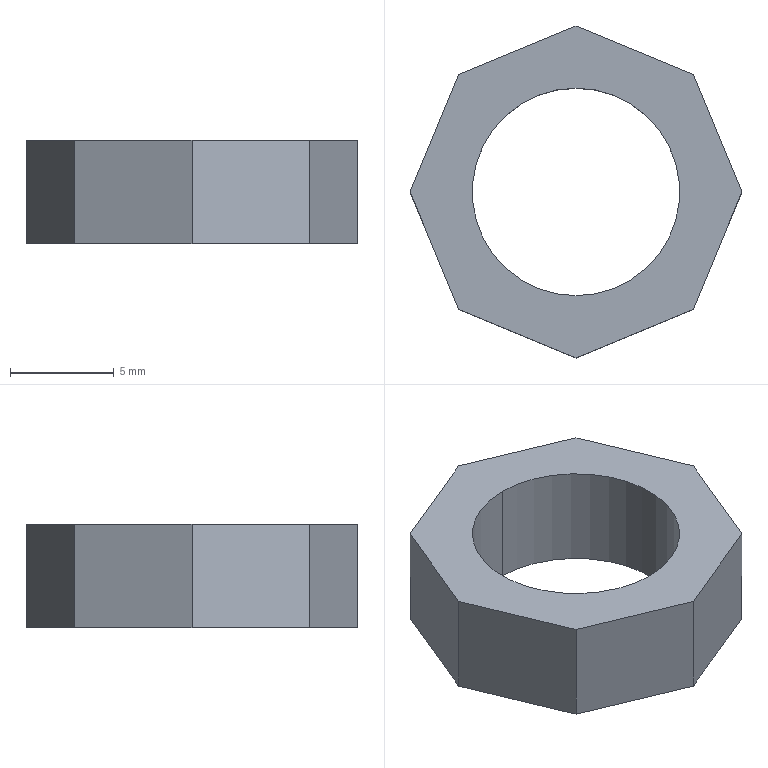Part | SolidWorks | features BaseBody 1 | 1 solid | 12 faces | box 16 x 16 x 5 mm | volume 512.398 mm3 | plane 10 | cylinder 2 | commonest cylinder face diameters 10 x2
STEP:
#1=CARTESIAN_POINT('',(-432.26,201.751,-430.));
#2=VERTEX_POINT('',#1);
#3=CARTESIAN_POINT('',(-432.26,211.751,-430.));
#4=VERTEX_POINT('',#3);
#5=CARTESIAN_POINT('',(-432.26,206.751,-430.));
#6=DIRECTION('',(0.,0.,1.));
#7=DIRECTION('',(0.,1.,0.));
#8=AXIS2_PLACEMENT_3D('',#5,#6,#7);
#9=CIRCLE('',#8,5.);
#10=EDGE_CURVE('',#2,#4,#9,.T.);
#11=ORIENTED_EDGE('',*,*,#10,.T.);
#12=CARTESIAN_POINT('',(-432.26,211.751,-435.));
#13=VERTEX_POINT('',#12);
#14=CARTESIAN_POINT('',(-432.26,211.751,-430.));
#15=DIRECTION('',(0.,0.,-1.));
#16=VECTOR('',#15,1000.);
#17=LINE('',#14,#16);
#18=EDGE_CURVE('',#4,#13,#17,.T.);
#19=ORIENTED_EDGE('',*,*,#18,.T.);
#20=CARTESIAN_POINT('',(-432.26,201.751,-435.));
#21=VERTEX_POINT('',#20);
#22=CARTESIAN_POINT('',(-432.26,206.751,-435.));
#23=DIRECTION('',(0.,0.,1.));
#24=DIRECTION('',(0.,1.,0.));
#25=AXIS2_PLACEMENT_3D('',#22,#23,#24);
#26=CIRCLE('',#25,5.);
#27=EDGE_CURVE('',#21,#13,#26,.T.);
#28=ORIENTED_EDGE('',*,*,#27,.F.);
#29=CARTESIAN_POINT('',(-432.26,201.751,-430.));
#30=DIRECTION('',(0.,0.,-1.));
#31=VECTOR('',#30,1000.);
#32=LINE('',#29,#31);
#33=EDGE_CURVE('',#2,#21,#32,.T.);
#34=ORIENTED_EDGE('',*,*,#33,.F.);
#35=EDGE_LOOP('',(#11,#19,#28,#34));
#36=FACE_OUTER_BOUND('',#35,.T.);
#37=CARTESIAN_POINT('',(-432.26,206.751,-430.));
#38=DIRECTION('',(0.,0.,-1.));
#39=DIRECTION('',(0.,-1.,0.));
#40=AXIS2_PLACEMENT_3D('',#37,#38,#39);
#41=CYLINDRICAL_SURFACE('',#40,5.);
#42=ADVANCED_FACE('',(#36),#41,.F.);
#43=CARTESIAN_POINT('',(-426.603,212.408,-430.));
#44=VERTEX_POINT('',#43);
#45=CARTESIAN_POINT('',(-432.26,214.751,-430.));
#46=VERTEX_POINT('',#45);
#47=CARTESIAN_POINT('',(-432.26,214.751,-430.));
#48=DIRECTION('',(-0.9239,0.3827,0.));
#49=VECTOR('',#48,1000.);
#50=LINE('',#47,#49);
#51=EDGE_CURVE('',#44,#46,#50,.T.);
#52=ORIENTED_EDGE('',*,*,#51,.T.);
#53=CARTESIAN_POINT('',(-437.917,212.408,-430.));
#54=VERTEX_POINT('',#53);
#55=CARTESIAN_POINT('',(-437.917,212.408,-430.));
#56=DIRECTION('',(-0.9239,-0.3827,0.));
#57=VECTOR('',#56,1000.);
#58=LINE('',#55,#57);
#59=EDGE_CURVE('',#46,#54,#58,.T.);
#60=ORIENTED_EDGE('',*,*,#59,.T.);
#61=CARTESIAN_POINT('',(-440.26,206.751,-430.));
#62=VERTEX_POINT('',#61);
#63=CARTESIAN_POINT('',(-440.26,206.751,-430.));
#64=DIRECTION('',(-0.3827,-0.9239,0.));
#65=VECTOR('',#64,1000.);
#66=LINE('',#63,#65);
#67=EDGE_CURVE('',#54,#62,#66,.T.);
#68=ORIENTED_EDGE('',*,*,#67,.T.);
#69=CARTESIAN_POINT('',(-437.917,201.094,-430.));
#70=VERTEX_POINT('',#69);
#71=CARTESIAN_POINT('',(-440.26,206.751,-430.));
#72=DIRECTION('',(0.3827,-0.9239,0.));
#73=VECTOR('',#72,1000.);
#74=LINE('',#71,#73);
#75=EDGE_CURVE('',#62,#70,#74,.T.);
#76=ORIENTED_EDGE('',*,*,#75,.T.);
#77=CARTESIAN_POINT('',(-432.26,198.751,-430.));
#78=VERTEX_POINT('',#77);
#79=CARTESIAN_POINT('',(-437.917,201.094,-430.));
#80=DIRECTION('',(0.9239,-0.3827,0.));
#81=VECTOR('',#80,1000.);
#82=LINE('',#79,#81);
#83=EDGE_CURVE('',#70,#78,#82,.T.);
#84=ORIENTED_EDGE('',*,*,#83,.T.);
#85=CARTESIAN_POINT('',(-426.603,201.094,-430.));
#86=VERTEX_POINT('',#85);
#87=CARTESIAN_POINT('',(-432.26,198.751,-430.));
#88=DIRECTION('',(0.9239,0.3827,0.));
#89=VECTOR('',#88,1000.);
#90=LINE('',#87,#89);
#91=EDGE_CURVE('',#78,#86,#90,.T.);
#92=ORIENTED_EDGE('',*,*,#91,.T.);
#93=CARTESIAN_POINT('',(-424.26,206.751,-430.));
#94=VERTEX_POINT('',#93);
#95=CARTESIAN_POINT('',(-426.603,201.094,-430.));
#96=DIRECTION('',(0.3827,0.9239,0.));
#97=VECTOR('',#96,1000.);
#98=LINE('',#95,#97);
#99=EDGE_CURVE('',#86,#94,#98,.T.);
#100=ORIENTED_EDGE('',*,*,#99,.T.);
#101=CARTESIAN_POINT('',(-426.603,212.408,-430.));
#102=DIRECTION('',(-0.3827,0.9239,0.));
#103=VECTOR('',#102,1000.);
#104=LINE('',#101,#103);
#105=EDGE_CURVE('',#94,#44,#104,.T.);
#106=ORIENTED_EDGE('',*,*,#105,.T.);
#107=EDGE_LOOP('',(#52,#60,#68,#76,#84,#92,#100,#106));
#108=FACE_OUTER_BOUND('',#107,.T.);
#109=ORIENTED_EDGE('',*,*,#10,.F.);
#110=CARTESIAN_POINT('',(-432.26,206.751,-430.));
#111=DIRECTION('',(0.,0.,1.));
#112=DIRECTION('',(0.,1.,0.));
#113=AXIS2_PLACEMENT_3D('',#110,#111,#112);
#114=CIRCLE('',#113,5.);
#115=EDGE_CURVE('',#4,#2,#114,.T.);
#116=ORIENTED_EDGE('',*,*,#115,.F.);
#117=EDGE_LOOP('',(#109,#116));
#118=FACE_BOUND('',#117,.T.);
#119=CARTESIAN_POINT('',(-432.26,206.751,-430.));
#120=DIRECTION('',(0.,0.,-1.));
#121=DIRECTION('',(0.,-1.,0.));
#122=AXIS2_PLACEMENT_3D('',#119,#120,#121);
#123=PLANE('',#122);
#124=ADVANCED_FACE('',(#108,#118),#123,.F.);
#125=CARTESIAN_POINT('',(-426.603,212.408,-435.));
#126=VERTEX_POINT('',#125);
#127=CARTESIAN_POINT('',(-432.26,214.751,-435.));
#128=VERTEX_POINT('',#127);
#129=CARTESIAN_POINT('',(-432.26,214.751,-435.));
#130=DIRECTION('',(-0.9239,0.3827,0.));
#131=VECTOR('',#130,1000.);
#132=LINE('',#129,#131);
#133=EDGE_CURVE('',#126,#128,#132,.T.);
#134=ORIENTED_EDGE('',*,*,#133,.F.);
#135=CARTESIAN_POINT('',(-424.26,206.751,-435.));
#136=VERTEX_POINT('',#135);
#137=CARTESIAN_POINT('',(-426.603,212.408,-435.));
#138=DIRECTION('',(-0.3827,0.9239,0.));
#139=VECTOR('',#138,1000.);
#140=LINE('',#137,#139);
#141=EDGE_CURVE('',#136,#126,#140,.T.);
#142=ORIENTED_EDGE('',*,*,#141,.F.);
#143=CARTESIAN_POINT('',(-426.603,201.094,-435.));
#144=VERTEX_POINT('',#143);
#145=CARTESIAN_POINT('',(-426.603,201.094,-435.));
#146=DIRECTION('',(0.3827,0.9239,0.));
#147=VECTOR('',#146,1000.);
#148=LINE('',#145,#147);
#149=EDGE_CURVE('',#144,#136,#148,.T.);
#150=ORIENTED_EDGE('',*,*,#149,.F.);
#151=CARTESIAN_POINT('',(-432.26,198.751,-435.));
#152=VERTEX_POINT('',#151);
#153=CARTESIAN_POINT('',(-432.26,198.751,-435.));
#154=DIRECTION('',(0.9239,0.3827,0.));
#155=VECTOR('',#154,1000.);
#156=LINE('',#153,#155);
#157=EDGE_CURVE('',#152,#144,#156,.T.);
#158=ORIENTED_EDGE('',*,*,#157,.F.);
#159=CARTESIAN_POINT('',(-437.917,201.094,-435.));
#160=VERTEX_POINT('',#159);
#161=CARTESIAN_POINT('',(-437.917,201.094,-435.));
#162=DIRECTION('',(0.9239,-0.3827,0.));
#163=VECTOR('',#162,1000.);
#164=LINE('',#161,#163);
#165=EDGE_CURVE('',#160,#152,#164,.T.);
#166=ORIENTED_EDGE('',*,*,#165,.F.);
#167=CARTESIAN_POINT('',(-440.26,206.751,-435.));
#168=VERTEX_POINT('',#167);
#169=CARTESIAN_POINT('',(-440.26,206.751,-435.));
#170=DIRECTION('',(0.3827,-0.9239,0.));
#171=VECTOR('',#170,1000.);
#172=LINE('',#169,#171);
#173=EDGE_CURVE('',#168,#160,#172,.T.);
#174=ORIENTED_EDGE('',*,*,#173,.F.);
#175=CARTESIAN_POINT('',(-437.917,212.408,-435.));
#176=VERTEX_POINT('',#175);
#177=CARTESIAN_POINT('',(-440.26,206.751,-435.));
#178=DIRECTION('',(-0.3827,-0.9239,0.));
#179=VECTOR('',#178,1000.);
#180=LINE('',#177,#179);
#181=EDGE_CURVE('',#176,#168,#180,.T.);
#182=ORIENTED_EDGE('',*,*,#181,.F.);
#183=CARTESIAN_POINT('',(-437.917,212.408,-435.));
#184=DIRECTION('',(-0.9239,-0.3827,0.));
#185=VECTOR('',#184,1000.);
#186=LINE('',#183,#185);
#187=EDGE_CURVE('',#128,#176,#186,.T.);
#188=ORIENTED_EDGE('',*,*,#187,.F.);
#189=EDGE_LOOP('',(#134,#142,#150,#158,#166,#174,#182,#188));
#190=FACE_OUTER_BOUND('',#189,.T.);
#191=ORIENTED_EDGE('',*,*,#27,.T.);
#192=CARTESIAN_POINT('',(-432.26,206.751,-435.));
#193=DIRECTION('',(0.,0.,1.));
#194=DIRECTION('',(0.,1.,0.));
#195=AXIS2_PLACEMENT_3D('',#192,#193,#194);
#196=CIRCLE('',#195,5.);
#197=EDGE_CURVE('',#13,#21,#196,.T.);
#198=ORIENTED_EDGE('',*,*,#197,.T.);
#199=EDGE_LOOP('',(#191,#198));
#200=FACE_BOUND('',#199,.T.);
#201=CARTESIAN_POINT('',(-432.26,206.751,-435.));
#202=DIRECTION('',(0.,0.,-1.));
#203=DIRECTION('',(0.,-1.,0.));
#204=AXIS2_PLACEMENT_3D('',#201,#202,#203);
#205=PLANE('',#204);
#206=ADVANCED_FACE('',(#190,#200),#205,.T.);
#207=ORIENTED_EDGE('',*,*,#133,.T.);
#208=CARTESIAN_POINT('',(-432.26,214.751,-430.));
#209=DIRECTION('',(0.,0.,1.));
#210=VECTOR('',#209,1000.);
#211=LINE('',#208,#210);
#212=EDGE_CURVE('',#128,#46,#211,.T.);
#213=ORIENTED_EDGE('',*,*,#212,.T.);
#214=ORIENTED_EDGE('',*,*,#51,.F.);
#215=CARTESIAN_POINT('',(-426.603,212.408,-430.));
#216=DIRECTION('',(0.,0.,1.));
#217=VECTOR('',#216,1000.);
#218=LINE('',#215,#217);
#219=EDGE_CURVE('',#126,#44,#218,.T.);
#220=ORIENTED_EDGE('',*,*,#219,.F.);
#221=EDGE_LOOP('',(#207,#213,#214,#220));
#222=FACE_OUTER_BOUND('',#221,.T.);
#223=CARTESIAN_POINT('',(-432.26,214.751,-430.));
#224=DIRECTION('',(-0.3827,-0.9239,0.));
#225=DIRECTION('',(-0.9239,0.3827,0.));
#226=AXIS2_PLACEMENT_3D('',#223,#224,#225);
#227=PLANE('',#226);
#228=ADVANCED_FACE('',(#222),#227,.F.);
#229=ORIENTED_EDGE('',*,*,#141,.T.);
#230=ORIENTED_EDGE('',*,*,#219,.T.);
#231=ORIENTED_EDGE('',*,*,#105,.F.);
#232=CARTESIAN_POINT('',(-424.26,206.751,-430.));
#233=DIRECTION('',(0.,0.,1.));
#234=VECTOR('',#233,1000.);
#235=LINE('',#232,#234);
#236=EDGE_CURVE('',#136,#94,#235,.T.);
#237=ORIENTED_EDGE('',*,*,#236,.F.);
#238=EDGE_LOOP('',(#229,#230,#231,#237));
#239=FACE_OUTER_BOUND('',#238,.T.);
#240=CARTESIAN_POINT('',(-426.603,212.408,-430.));
#241=DIRECTION('',(-0.9239,-0.3827,0.));
#242=DIRECTION('',(-0.3827,0.9239,0.));
#243=AXIS2_PLACEMENT_3D('',#240,#241,#242);
#244=PLANE('',#243);
#245=ADVANCED_FACE('',(#239),#244,.F.);
#246=ORIENTED_EDGE('',*,*,#149,.T.);
#247=ORIENTED_EDGE('',*,*,#236,.T.);
#248=ORIENTED_EDGE('',*,*,#99,.F.);
#249=CARTESIAN_POINT('',(-426.603,201.094,-430.));
#250=DIRECTION('',(0.,0.,1.));
#251=VECTOR('',#250,1000.);
#252=LINE('',#249,#251);
#253=EDGE_CURVE('',#144,#86,#252,.T.);
#254=ORIENTED_EDGE('',*,*,#253,.F.);
#255=EDGE_LOOP('',(#246,#247,#248,#254));
#256=FACE_OUTER_BOUND('',#255,.T.);
#257=CARTESIAN_POINT('',(-426.603,201.094,-430.));
#258=DIRECTION('',(-0.9239,0.3827,0.));
#259=DIRECTION('',(0.3827,0.9239,0.));
#260=AXIS2_PLACEMENT_3D('',#257,#258,#259);
#261=PLANE('',#260);
#262=ADVANCED_FACE('',(#256),#261,.F.);
#263=ORIENTED_EDGE('',*,*,#157,.T.);
#264=ORIENTED_EDGE('',*,*,#253,.T.);
#265=ORIENTED_EDGE('',*,*,#91,.F.);
#266=CARTESIAN_POINT('',(-432.26,198.751,-430.));
#267=DIRECTION('',(0.,0.,1.));
#268=VECTOR('',#267,1000.);
#269=LINE('',#266,#268);
#270=EDGE_CURVE('',#152,#78,#269,.T.);
#271=ORIENTED_EDGE('',*,*,#270,.F.);
#272=EDGE_LOOP('',(#263,#264,#265,#271));
#273=FACE_OUTER_BOUND('',#272,.T.);
#274=CARTESIAN_POINT('',(-432.26,198.751,-430.));
#275=DIRECTION('',(-0.3827,0.9239,0.));
#276=DIRECTION('',(0.9239,0.3827,0.));
#277=AXIS2_PLACEMENT_3D('',#274,#275,#276);
#278=PLANE('',#277);
#279=ADVANCED_FACE('',(#273),#278,.F.);
#280=ORIENTED_EDGE('',*,*,#165,.T.);
#281=ORIENTED_EDGE('',*,*,#270,.T.);
#282=ORIENTED_EDGE('',*,*,#83,.F.);
#283=CARTESIAN_POINT('',(-437.917,201.094,-430.));
#284=DIRECTION('',(0.,0.,1.));
#285=VECTOR('',#284,1000.);
#286=LINE('',#283,#285);
#287=EDGE_CURVE('',#160,#70,#286,.T.);
#288=ORIENTED_EDGE('',*,*,#287,.F.);
#289=EDGE_LOOP('',(#280,#281,#282,#288));
#290=FACE_OUTER_BOUND('',#289,.T.);
#291=CARTESIAN_POINT('',(-437.917,201.094,-430.));
#292=DIRECTION('',(0.3827,0.9239,0.));
#293=DIRECTION('',(0.9239,-0.3827,0.));
#294=AXIS2_PLACEMENT_3D('',#291,#292,#293);
#295=PLANE('',#294);
#296=ADVANCED_FACE('',(#290),#295,.F.);
#297=ORIENTED_EDGE('',*,*,#173,.T.);
#298=ORIENTED_EDGE('',*,*,#287,.T.);
#299=ORIENTED_EDGE('',*,*,#75,.F.);
#300=CARTESIAN_POINT('',(-440.26,206.751,-430.));
#301=DIRECTION('',(0.,0.,1.));
#302=VECTOR('',#301,1000.);
#303=LINE('',#300,#302);
#304=EDGE_CURVE('',#168,#62,#303,.T.);
#305=ORIENTED_EDGE('',*,*,#304,.F.);
#306=EDGE_LOOP('',(#297,#298,#299,#305));
#307=FACE_OUTER_BOUND('',#306,.T.);
#308=CARTESIAN_POINT('',(-440.26,206.751,-430.));
#309=DIRECTION('',(0.9239,0.3827,0.));
#310=DIRECTION('',(0.3827,-0.9239,0.));
#311=AXIS2_PLACEMENT_3D('',#308,#309,#310);
#312=PLANE('',#311);
#313=ADVANCED_FACE('',(#307),#312,.F.);
#314=ORIENTED_EDGE('',*,*,#181,.T.);
#315=ORIENTED_EDGE('',*,*,#304,.T.);
#316=ORIENTED_EDGE('',*,*,#67,.F.);
#317=CARTESIAN_POINT('',(-437.917,212.408,-430.));
#318=DIRECTION('',(0.,0.,1.));
#319=VECTOR('',#318,1000.);
#320=LINE('',#317,#319);
#321=EDGE_CURVE('',#176,#54,#320,.T.);
#322=ORIENTED_EDGE('',*,*,#321,.F.);
#323=EDGE_LOOP('',(#314,#315,#316,#322));
#324=FACE_OUTER_BOUND('',#323,.T.);
#325=CARTESIAN_POINT('',(-440.26,206.751,-430.));
#326=DIRECTION('',(0.9239,-0.3827,0.));
#327=DIRECTION('',(-0.3827,-0.9239,0.));
#328=AXIS2_PLACEMENT_3D('',#325,#326,#327);
#329=PLANE('',#328);
#330=ADVANCED_FACE('',(#324),#329,.F.);
#331=ORIENTED_EDGE('',*,*,#187,.T.);
#332=ORIENTED_EDGE('',*,*,#321,.T.);
#333=ORIENTED_EDGE('',*,*,#59,.F.);
#334=ORIENTED_EDGE('',*,*,#212,.F.);
#335=EDGE_LOOP('',(#331,#332,#333,#334));
#336=FACE_OUTER_BOUND('',#335,.T.);
#337=CARTESIAN_POINT('',(-437.917,212.408,-430.));
#338=DIRECTION('',(0.3827,-0.9239,0.));
#339=DIRECTION('',(-0.9239,-0.3827,0.));
#340=AXIS2_PLACEMENT_3D('',#337,#338,#339);
#341=PLANE('',#340);
#342=ADVANCED_FACE('',(#336),#341,.F.);
#343=ORIENTED_EDGE('',*,*,#18,.F.);
#344=ORIENTED_EDGE('',*,*,#115,.T.);
#345=ORIENTED_EDGE('',*,*,#33,.T.);
#346=ORIENTED_EDGE('',*,*,#197,.F.);
#347=EDGE_LOOP('',(#343,#344,#345,#346));
#348=FACE_OUTER_BOUND('',#347,.T.);
#349=CARTESIAN_POINT('',(-432.26,206.751,-430.));
#350=DIRECTION('',(0.,0.,-1.));
#351=DIRECTION('',(0.,-1.,0.));
#352=AXIS2_PLACEMENT_3D('',#349,#350,#351);
#353=CYLINDRICAL_SURFACE('',#352,5.);
#354=ADVANCED_FACE('',(#348),#353,.F.);
#355=CLOSED_SHELL('',(#42,#124,#206,#228,#245,#262,#279,#296,#313,#330,#342,#354));
#356=MANIFOLD_SOLID_BREP('',#355);
#357=CARTESIAN_POINT('',(0.,0.,0.));
#358=DIRECTION('',(0.,0.,1.));
#359=DIRECTION('',(1.,0.,0.));
#360=AXIS2_PLACEMENT_3D('',#357,#358,#359);
#361=(LENGTH_UNIT()NAMED_UNIT(*)SI_UNIT(.MILLI.,.METRE.));
#362=UNCERTAINTY_MEASURE_WITH_UNIT(LENGTH_MEASURE(0.00001),#361,'','');
#363=(NAMED_UNIT(*)PLANE_ANGLE_UNIT()SI_UNIT($,.RADIAN.));
#364=(NAMED_UNIT(*)SI_UNIT($,.STERADIAN.)SOLID_ANGLE_UNIT());
#365=(GEOMETRIC_REPRESENTATION_CONTEXT(3)GLOBAL_UNCERTAINTY_ASSIGNED_CONTEXT((#362))GLOBAL_UNIT_ASSIGNED_CONTEXT((#361,#363,#364))REPRESENTATION_CONTEXT('',''));
#366=ADVANCED_BREP_SHAPE_REPRESENTATION('',(#356,#360),#365);